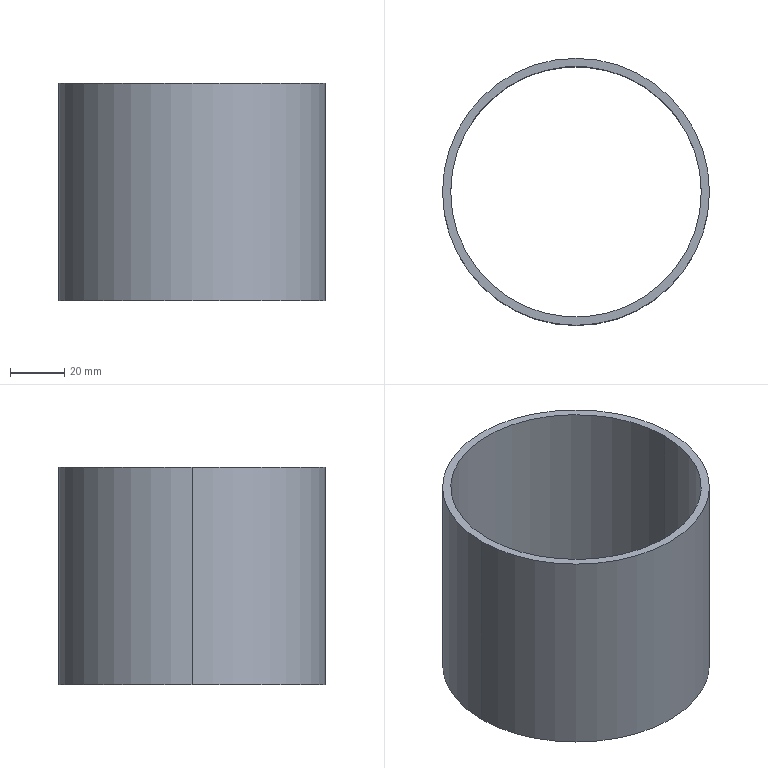Part | SolidWorks | features MirrorStock 1 | 1 solid | 6 faces | box 98 x 98 x 80 mm | volume 71628 mm3 | cylinder 4 | plane 2 | commonest cylinder face diameters 92 x2 98 x2
STEP:
#1=CARTESIAN_POINT('',(46.,0.,-40.));
#2=VERTEX_POINT('',#1);
#3=CARTESIAN_POINT('',(-46.,0.,-40.));
#4=VERTEX_POINT('',#3);
#5=CARTESIAN_POINT('',(0.,0.,-40.));
#6=DIRECTION('',(0.,0.,1.));
#7=DIRECTION('',(1.,0.,0.));
#8=AXIS2_PLACEMENT_3D('',#5,#6,#7);
#9=CIRCLE('',#8,46.);
#10=EDGE_CURVE('',#2,#4,#9,.T.);
#11=ORIENTED_EDGE('',*,*,#10,.F.);
#12=CARTESIAN_POINT('',(46.,0.,40.));
#13=VERTEX_POINT('',#12);
#14=CARTESIAN_POINT('',(46.,0.,-40.));
#15=DIRECTION('',(0.,0.,1.));
#16=VECTOR('',#15,1000.);
#17=LINE('',#14,#16);
#18=EDGE_CURVE('',#2,#13,#17,.T.);
#19=ORIENTED_EDGE('',*,*,#18,.T.);
#20=CARTESIAN_POINT('',(-46.,0.,40.));
#21=VERTEX_POINT('',#20);
#22=CARTESIAN_POINT('',(0.,0.,40.));
#23=DIRECTION('',(0.,0.,1.));
#24=DIRECTION('',(1.,0.,0.));
#25=AXIS2_PLACEMENT_3D('',#22,#23,#24);
#26=CIRCLE('',#25,46.);
#27=EDGE_CURVE('',#13,#21,#26,.T.);
#28=ORIENTED_EDGE('',*,*,#27,.T.);
#29=CARTESIAN_POINT('',(-46.,0.,-40.));
#30=DIRECTION('',(0.,0.,1.));
#31=VECTOR('',#30,1000.);
#32=LINE('',#29,#31);
#33=EDGE_CURVE('',#4,#21,#32,.T.);
#34=ORIENTED_EDGE('',*,*,#33,.F.);
#35=EDGE_LOOP('',(#11,#19,#28,#34));
#36=FACE_OUTER_BOUND('',#35,.T.);
#37=CARTESIAN_POINT('',(0.,0.,-40.));
#38=DIRECTION('',(0.,0.,1.));
#39=DIRECTION('',(-1.,0.,0.));
#40=AXIS2_PLACEMENT_3D('',#37,#38,#39);
#41=CYLINDRICAL_SURFACE('',#40,46.);
#42=ADVANCED_FACE('',(#36),#41,.F.);
#43=CARTESIAN_POINT('',(-49.,0.,-40.));
#44=VERTEX_POINT('',#43);
#45=CARTESIAN_POINT('',(49.,0.,-40.));
#46=VERTEX_POINT('',#45);
#47=CARTESIAN_POINT('',(0.,0.,-40.));
#48=DIRECTION('',(0.,0.,1.));
#49=DIRECTION('',(1.,0.,0.));
#50=AXIS2_PLACEMENT_3D('',#47,#48,#49);
#51=CIRCLE('',#50,49.);
#52=EDGE_CURVE('',#44,#46,#51,.T.);
#53=ORIENTED_EDGE('',*,*,#52,.T.);
#54=CARTESIAN_POINT('',(49.,0.,40.));
#55=VERTEX_POINT('',#54);
#56=CARTESIAN_POINT('',(49.,0.,-40.));
#57=DIRECTION('',(0.,0.,1.));
#58=VECTOR('',#57,1000.);
#59=LINE('',#56,#58);
#60=EDGE_CURVE('',#46,#55,#59,.T.);
#61=ORIENTED_EDGE('',*,*,#60,.T.);
#62=CARTESIAN_POINT('',(-49.,0.,40.));
#63=VERTEX_POINT('',#62);
#64=CARTESIAN_POINT('',(0.,0.,40.));
#65=DIRECTION('',(0.,0.,1.));
#66=DIRECTION('',(1.,0.,0.));
#67=AXIS2_PLACEMENT_3D('',#64,#65,#66);
#68=CIRCLE('',#67,49.);
#69=EDGE_CURVE('',#63,#55,#68,.T.);
#70=ORIENTED_EDGE('',*,*,#69,.F.);
#71=CARTESIAN_POINT('',(-49.,0.,-40.));
#72=DIRECTION('',(0.,0.,1.));
#73=VECTOR('',#72,1000.);
#74=LINE('',#71,#73);
#75=EDGE_CURVE('',#44,#63,#74,.T.);
#76=ORIENTED_EDGE('',*,*,#75,.F.);
#77=EDGE_LOOP('',(#53,#61,#70,#76));
#78=FACE_OUTER_BOUND('',#77,.T.);
#79=CARTESIAN_POINT('',(0.,0.,-40.));
#80=DIRECTION('',(0.,0.,1.));
#81=DIRECTION('',(-1.,0.,0.));
#82=AXIS2_PLACEMENT_3D('',#79,#80,#81);
#83=CYLINDRICAL_SURFACE('',#82,49.);
#84=ADVANCED_FACE('',(#78),#83,.T.);
#85=ORIENTED_EDGE('',*,*,#52,.F.);
#86=CARTESIAN_POINT('',(0.,0.,-40.));
#87=DIRECTION('',(0.,0.,1.));
#88=DIRECTION('',(1.,0.,0.));
#89=AXIS2_PLACEMENT_3D('',#86,#87,#88);
#90=CIRCLE('',#89,49.);
#91=EDGE_CURVE('',#46,#44,#90,.T.);
#92=ORIENTED_EDGE('',*,*,#91,.F.);
#93=EDGE_LOOP('',(#85,#92));
#94=FACE_OUTER_BOUND('',#93,.T.);
#95=CARTESIAN_POINT('',(0.,0.,-40.));
#96=DIRECTION('',(0.,0.,1.));
#97=DIRECTION('',(1.,0.,0.));
#98=AXIS2_PLACEMENT_3D('',#95,#96,#97);
#99=CIRCLE('',#98,46.);
#100=EDGE_CURVE('',#4,#2,#99,.T.);
#101=ORIENTED_EDGE('',*,*,#100,.T.);
#102=ORIENTED_EDGE('',*,*,#10,.T.);
#103=EDGE_LOOP('',(#101,#102));
#104=FACE_BOUND('',#103,.T.);
#105=CARTESIAN_POINT('',(0.,0.,-40.));
#106=DIRECTION('',(0.,0.,-1.));
#107=DIRECTION('',(1.,0.,0.));
#108=AXIS2_PLACEMENT_3D('',#105,#106,#107);
#109=PLANE('',#108);
#110=ADVANCED_FACE('',(#94,#104),#109,.T.);
#111=ORIENTED_EDGE('',*,*,#69,.T.);
#112=CARTESIAN_POINT('',(0.,0.,40.));
#113=DIRECTION('',(0.,0.,1.));
#114=DIRECTION('',(1.,0.,0.));
#115=AXIS2_PLACEMENT_3D('',#112,#113,#114);
#116=CIRCLE('',#115,49.);
#117=EDGE_CURVE('',#55,#63,#116,.T.);
#118=ORIENTED_EDGE('',*,*,#117,.T.);
#119=EDGE_LOOP('',(#111,#118));
#120=FACE_OUTER_BOUND('',#119,.T.);
#121=CARTESIAN_POINT('',(0.,0.,40.));
#122=DIRECTION('',(0.,0.,1.));
#123=DIRECTION('',(1.,0.,0.));
#124=AXIS2_PLACEMENT_3D('',#121,#122,#123);
#125=CIRCLE('',#124,46.);
#126=EDGE_CURVE('',#21,#13,#125,.T.);
#127=ORIENTED_EDGE('',*,*,#126,.F.);
#128=ORIENTED_EDGE('',*,*,#27,.F.);
#129=EDGE_LOOP('',(#127,#128));
#130=FACE_BOUND('',#129,.T.);
#131=CARTESIAN_POINT('',(0.,0.,40.));
#132=DIRECTION('',(0.,0.,-1.));
#133=DIRECTION('',(1.,0.,0.));
#134=AXIS2_PLACEMENT_3D('',#131,#132,#133);
#135=PLANE('',#134);
#136=ADVANCED_FACE('',(#120,#130),#135,.F.);
#137=ORIENTED_EDGE('',*,*,#60,.F.);
#138=ORIENTED_EDGE('',*,*,#91,.T.);
#139=ORIENTED_EDGE('',*,*,#75,.T.);
#140=ORIENTED_EDGE('',*,*,#117,.F.);
#141=EDGE_LOOP('',(#137,#138,#139,#140));
#142=FACE_OUTER_BOUND('',#141,.T.);
#143=CARTESIAN_POINT('',(0.,0.,-40.));
#144=DIRECTION('',(0.,0.,1.));
#145=DIRECTION('',(-1.,0.,0.));
#146=AXIS2_PLACEMENT_3D('',#143,#144,#145);
#147=CYLINDRICAL_SURFACE('',#146,49.);
#148=ADVANCED_FACE('',(#142),#147,.T.);
#149=ORIENTED_EDGE('',*,*,#18,.F.);
#150=ORIENTED_EDGE('',*,*,#100,.F.);
#151=ORIENTED_EDGE('',*,*,#33,.T.);
#152=ORIENTED_EDGE('',*,*,#126,.T.);
#153=EDGE_LOOP('',(#149,#150,#151,#152));
#154=FACE_OUTER_BOUND('',#153,.T.);
#155=CARTESIAN_POINT('',(0.,0.,-40.));
#156=DIRECTION('',(0.,0.,1.));
#157=DIRECTION('',(-1.,0.,0.));
#158=AXIS2_PLACEMENT_3D('',#155,#156,#157);
#159=CYLINDRICAL_SURFACE('',#158,46.);
#160=ADVANCED_FACE('',(#154),#159,.F.);
#161=CLOSED_SHELL('',(#42,#84,#110,#136,#148,#160));
#162=MANIFOLD_SOLID_BREP('',#161);
#163=CARTESIAN_POINT('',(0.,0.,0.));
#164=DIRECTION('',(0.,0.,1.));
#165=DIRECTION('',(1.,0.,0.));
#166=AXIS2_PLACEMENT_3D('',#163,#164,#165);
#167=(LENGTH_UNIT()NAMED_UNIT(*)SI_UNIT(.MILLI.,.METRE.));
#168=UNCERTAINTY_MEASURE_WITH_UNIT(LENGTH_MEASURE(0.00001),#167,'','');
#169=(NAMED_UNIT(*)PLANE_ANGLE_UNIT()SI_UNIT($,.RADIAN.));
#170=(NAMED_UNIT(*)SI_UNIT($,.STERADIAN.)SOLID_ANGLE_UNIT());
#171=(GEOMETRIC_REPRESENTATION_CONTEXT(3)GLOBAL_UNCERTAINTY_ASSIGNED_CONTEXT((#168))GLOBAL_UNIT_ASSIGNED_CONTEXT((#167,#169,#170))REPRESENTATION_CONTEXT('',''));
#172=ADVANCED_BREP_SHAPE_REPRESENTATION('',(#162,#166),#171);